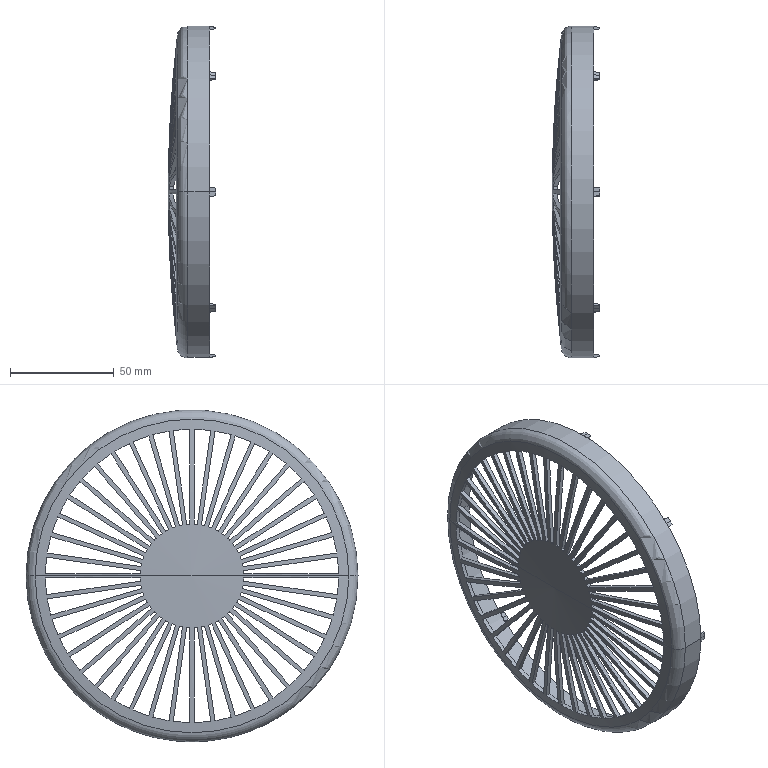Part | SolidWorks | features ICE 2, CirPattern 1, Fillet 1, Revolution 1, Shell 1 | 1 solid | 245 faces | box 23 x 160 x 160 mm | volume 32777 mm3 | plane 113 | cylinder 92 | cone 32 | torus 4 | sphere 4 | commonest cylinder face diameters 50 x44 141.176 x44 156 x2 160 x2